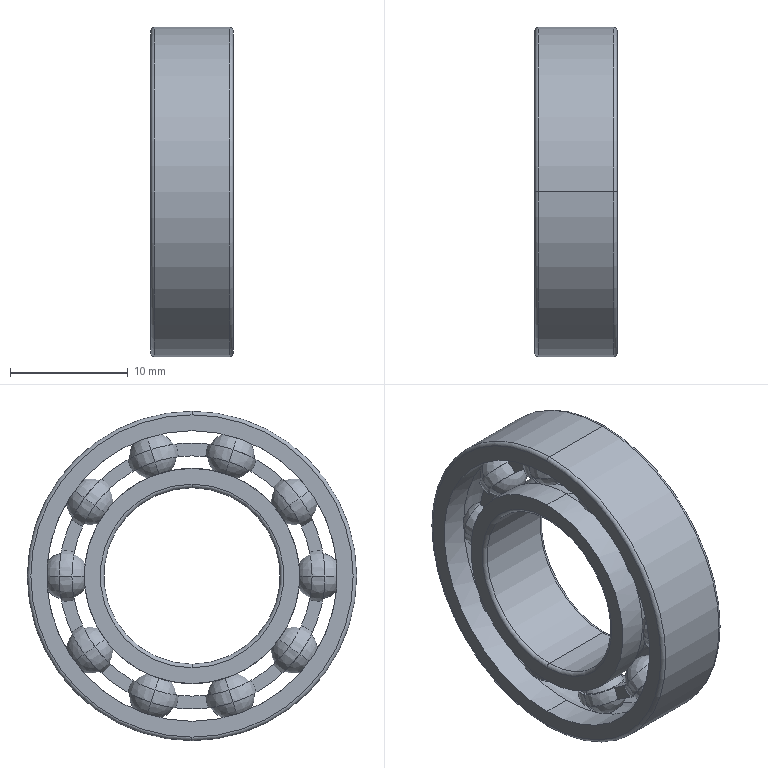Part | SolidWorks | features Revolution 5, CirPattern 2, RevCut 2 | 1 solid | 161 faces | box 7 x 28 x 28 mm | volume 1855 mm3 | sphere 80 | torus 41 | plane 24 | cylinder 16 | commonest cylinder face diameters 18.3 x4 24.7 x4 15 x2 20.409 x2 22.591 x2 28 x2